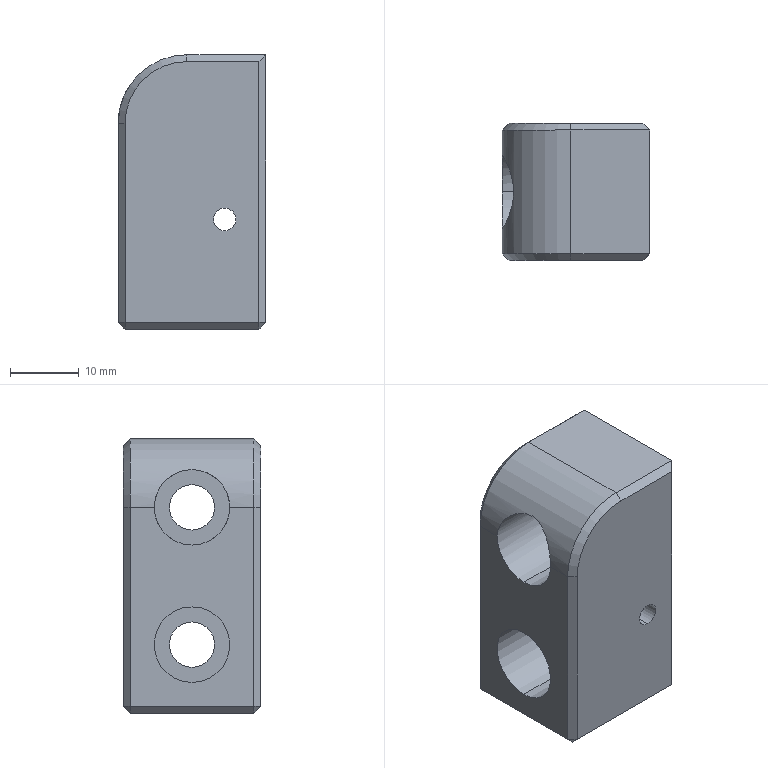Part | STEP file | 1 solid | 42 faces | box 21.5 x 20 x 40 mm | volume 13498 mm3 | plane 23 | cylinder 15 | cone 4 | commonest cylinder face diameters 3.3 x4 6.6 x4 11 x4 8.1 x2 20 x1